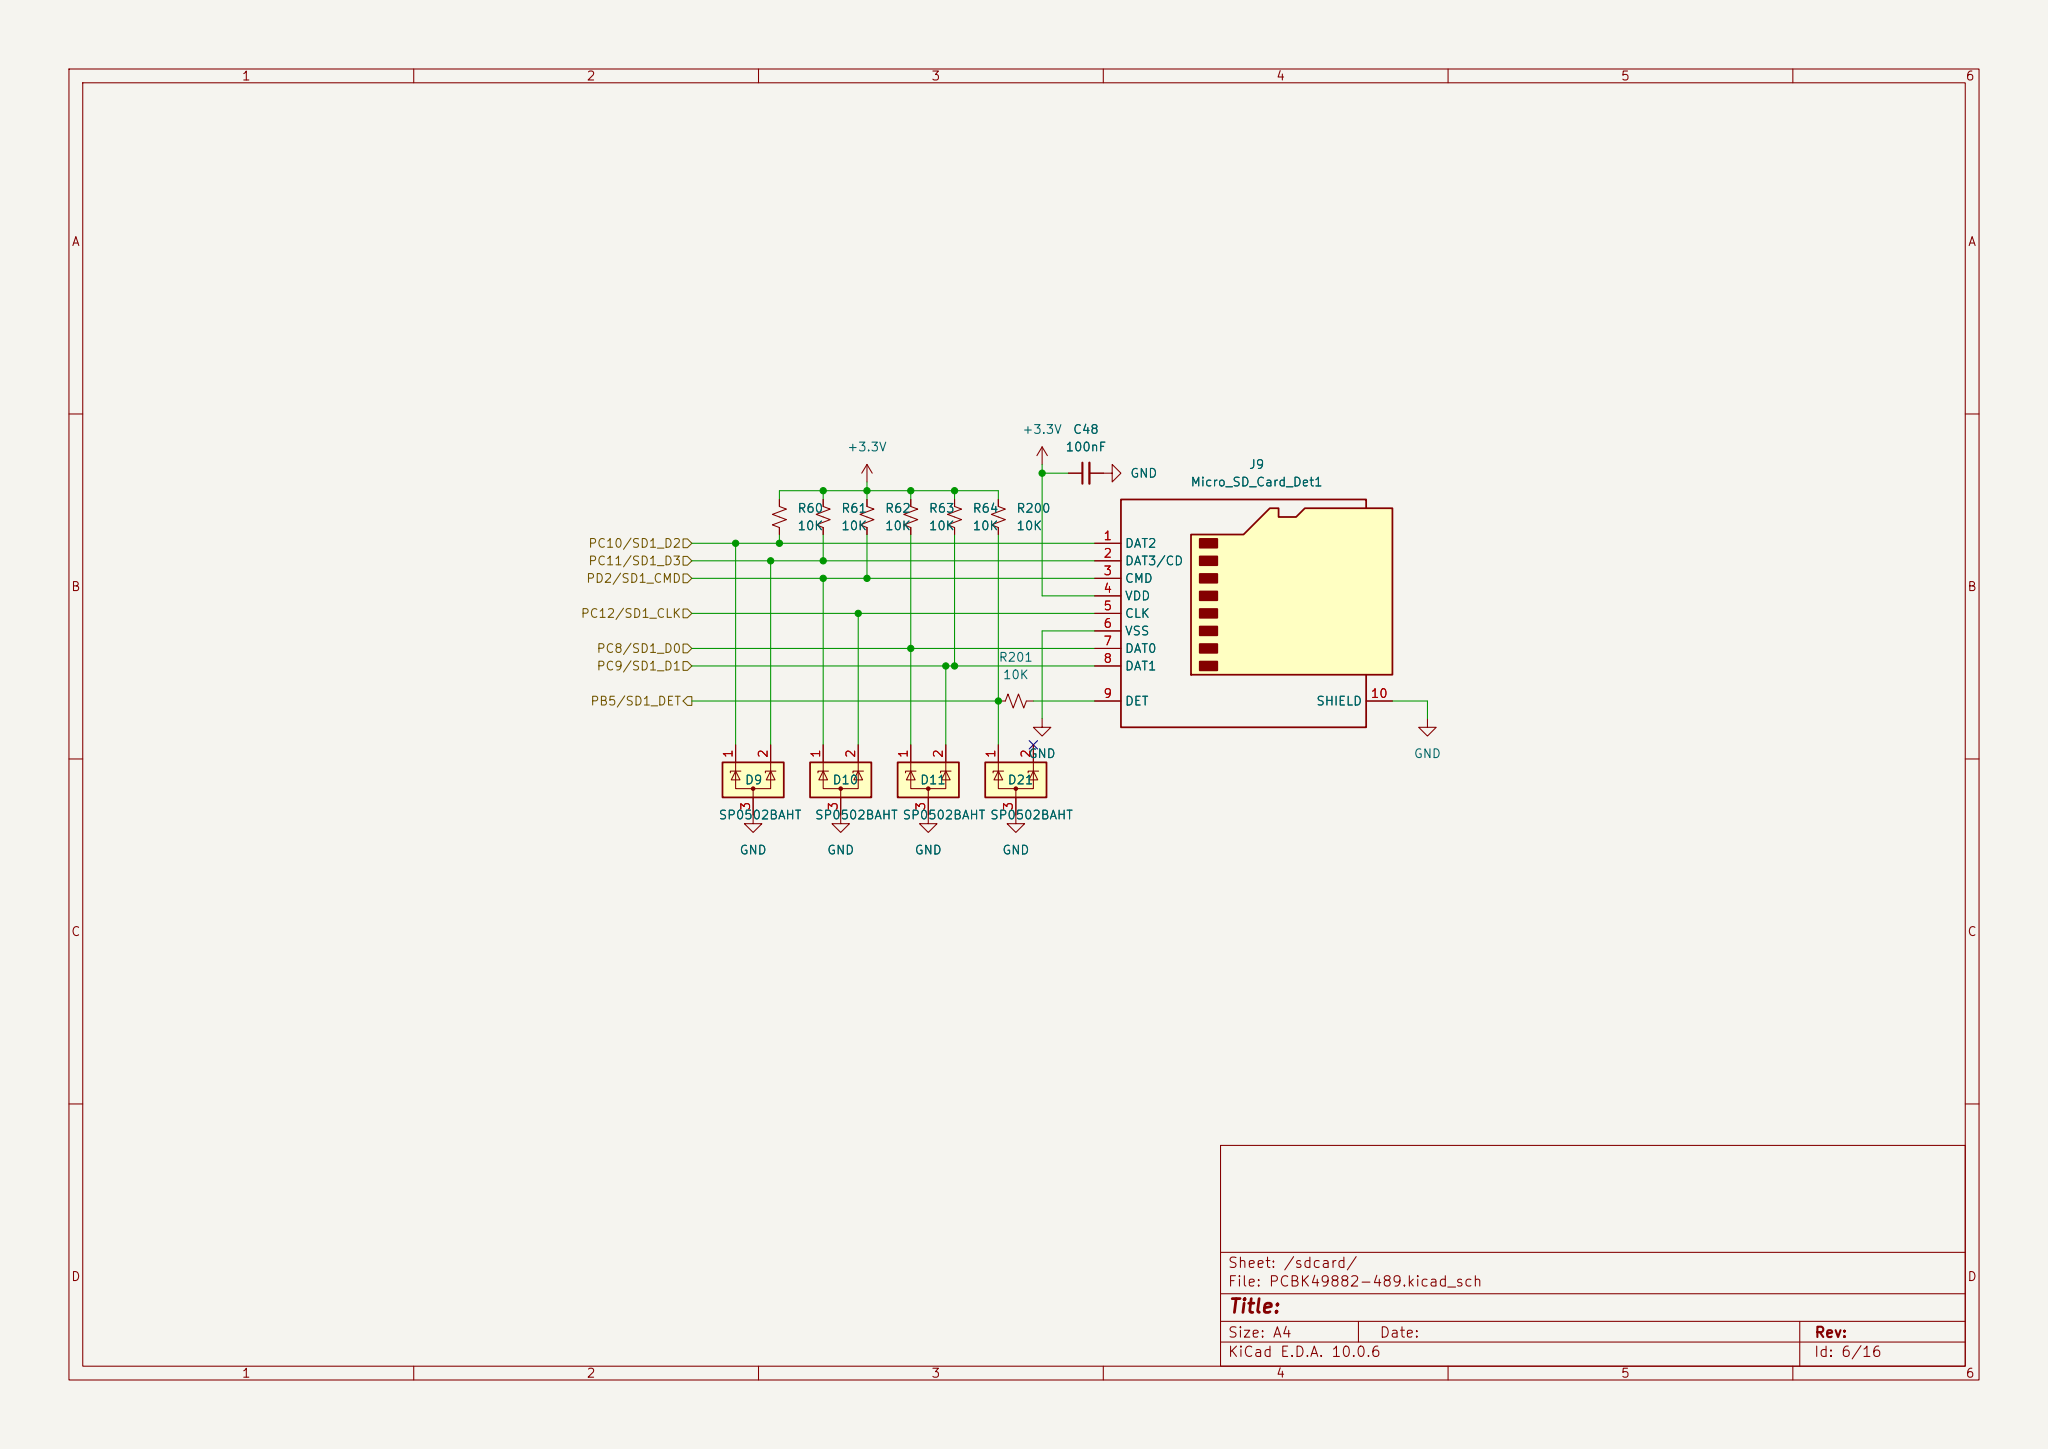Circuit board | KiCad | 536 parts | 438 nets | one sheet of the schematic
Parts on this sheet (reference | value | footprint):
C48 | 100nF | Capacitor_SMD:C_0603_1608Metric
D10
D11
D21 | SP0502BAHT | Package_TO_SOT_SMD:SOT-23
D9
J9 | Micro_SD_Card_Det1 | Connector_User:TF-PUSH
R200
R201
R60
R61
R62
R63
R64
Nets of these parts (net: part-pin ...):
+3.3V: C48-1 J9-4 R60-1 R61-1 R62-1 R63-1 R64-1 R200-1
/core_board_b2b/PB5{slash}SD1_DET: D21-1 R200-2 R201-1
/core_board_b2b/PC8{slash}SD1_D0: D11-1 J9-7 R63-2
/core_board_b2b/PC9{slash}SD1_D1: D11-2 J9-8 R64-2
/core_board_b2b/PC10{slash}SD1_D2: D9-1 J9-1 R60-2
/core_board_b2b/PC11{slash}SD1_D3: D9-2 J9-2 R61-2
/core_board_b2b/PC12{slash}SD1_CLK: D10-2 J9-5
/core_board_b2b/PD2{slash}SD1_CMD: D10-1 J9-3 R62-2
GND: C48-2 D9-3 D10-3 D11-3 D21-3 J9-6 J9-10 J9-11 J9-12 J9-13
Net-(J9-DET): J9-9 R201-2
unconnected-(D21-K-Pad2): D21-2